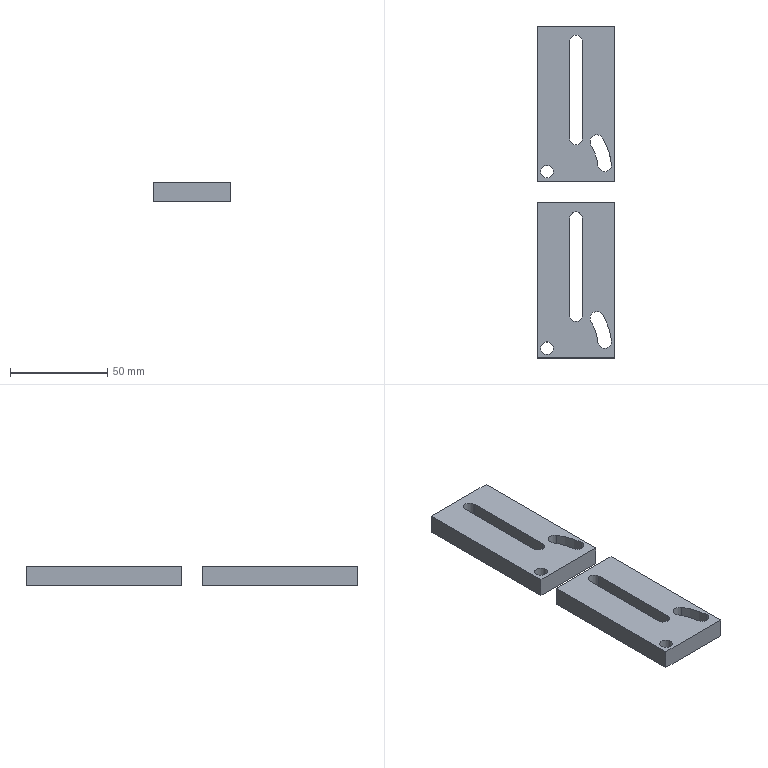CAM job | NX | 3-axis milling, drilling | part box 40 x 171 x 10 mm | stock box 45 x 176 x 12 mm
Tools:
number,name,description,diameter,corner_radius,flute_length,length,flutes
4,D4,平底铣刀-粗,4.0,0.0,25.0,75.0,2
6,D6,平底铣刀-粗,6.0,0.0,25.0,75.0,2
9,D10,平底铣刀-粗,10.0,0.0,35.0,75.0,2
11,D4-J,平底铣刀-精,4.0,0.0,50.0,75.0,2
10,D10-J,平底铣刀-精,10.0,0.0,35.0,75.0,2
1,D80R0.8飞刀,圆鼻刀-粗,80.0,0.8,50.0,75.0,2
1,D80R0.8飞刀-J,圆鼻刀-精,80.0,0.8,50.0,75.0,2
2,D6倒角刀,倒角刀,6.0,0.0,3.0,25.0,2
17,ZT6.5,钻头,6.5,0.0,35.0,50.0,2
Operations:
program,operation,operation_type,tool,method,geometry_group,spindle_rpm,surface_speed,feed_per_tooth,feed_cut,feed_plunge,cut_length_mm,path_length_mm,cut_time_min,machine_time_min
B,底壁铣飞面一刀开粗_COPY,VolumeBased25DMillingOperation,D80R0.8飞刀,分层开粗-切深K-步距G,W-B,2800.0,703.696,0.5357,3000.0,100.0,1116.776,1976.734,0.3723,0.4583
B,底壁铣飞面一刀精光_COPY,VolumeBased25DMillingOperation,D80R0.8飞刀-J,侧刃精光-切深K-步距G,W-B,4000.0,1005.28,0.125,1000.0,100.0,278.998,314.998,0.279,0.2826
B,平面去毛刺6X45L_COPY,SurfaceContour,D6倒角刀,爬面_倒角-切深0-步距G,W-B,6500.0,122.519,0.1154,1500.0,100.0,861.067,1295.441,0.574,0.6175
A,顶面,FaceMilling,D80R0.8飞刀,侧刃精光-切深K-步距G,W-A,4000.0,1005.31,0.125,1000.0,100.0,265.0,301.0,0.265,0.2686
A,外形粗_2,VolumeBased25DMillingOperation,D10,METHOD,W-A,8000.0,251.327,0.3125,5000.0,80.0,8164.356,8351.856,1.633,1.652
A,打点-深0.8,Operation,D6倒角刀,NONE,W-A,8000.0,150.796,0.0312,500.0,90.0,3.6,139.206,0.0072,0.0208
A,通孔-6-8,Operation,ZT6.5,NONE,W-A,2500.0,51.051,0.03,150.0,90.0,29.906,191.817,0.1994,0.2156
A,腰槽粗_1,VolumeBased25DMillingOperation,D6,METHOD,W-A,6000.0,113.0,0.2083,2500.0,100.0,1569.905,1751.123,0.628,0.6461
A,通腰槽粗_1,VolumeBased25DMillingOperation,D4,METHOD,W-A,6000.0,75.398,0.1,1200.0,100.0,9438.883,9627.812,7.866,7.885
A,腰槽精_1,VolumeBased25DMillingOperation,D4-J,METHOD,W-A,6000.0,113.0,0.0417,500.0,100.0,660.494,905.994,1.321,1.345
A,腰槽精_2,VolumeBased25DMillingOperation,D4-J,METHOD,W-A,6000.0,113.0,0.0667,800.0,100.0,148.475,381.583,0.1856,0.2089
A,仅选体,SurfaceContour,D6倒角刀,METHOD,W-A,8000.0,150.796,0.1875,3000.0,100.0,854.355,1289.441,0.2848,0.3283
A,铣倒角_1,PlanarMilling,D6倒角刀,METHOD,W-A,8000.0,150.796,0.05,800.0,100.0,46.107,222.107,0.0576,0.0752
A,外形半精_2,VolumeBased25DMillingOperation,D10-J,METHOD,W-A,8000.0,251.327,0.0625,1000.0,100.0,560.903,619.903,0.5609,0.5668